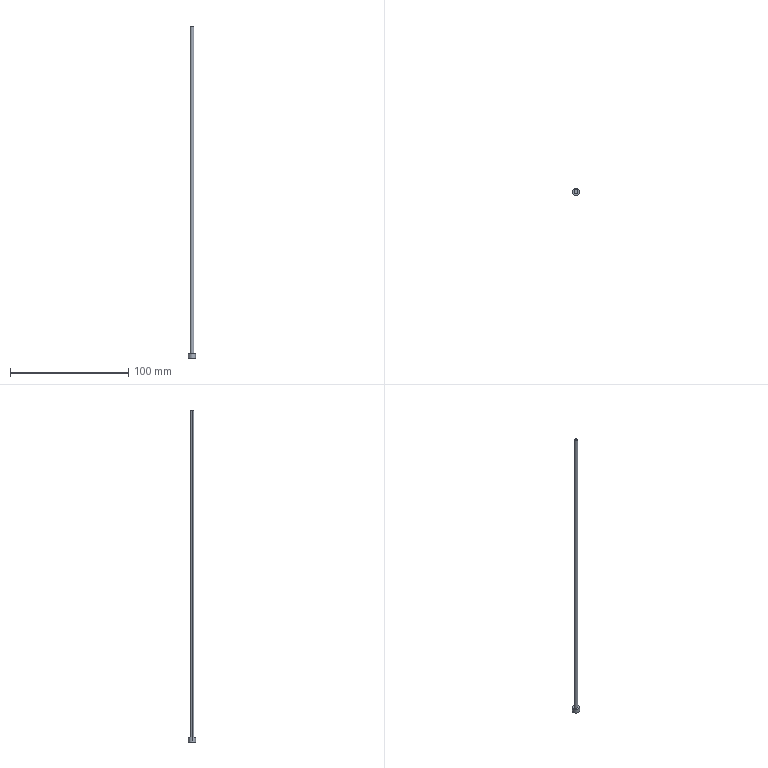Part | Creo | 1 solid | 7 faces | box 6 x 6 x 280.196 mm | volume 2065 mm3 | cylinder 4 | plane 3 | commonest cylinder face diameters 3 x2 6 x2
STEP:
#1=CARTESIAN_POINT('',(-83.5,0.,-292.));
#2=VERTEX_POINT('',#1);
#3=CARTESIAN_POINT('',(-86.5,0.,-292.));
#4=VERTEX_POINT('',#3);
#5=CARTESIAN_POINT('',(-85.,0.,-292.));
#6=DIRECTION('',(0.,0.,-1.));
#7=DIRECTION('',(1.,0.,0.));
#8=AXIS2_PLACEMENT_3D('',#5,#6,#7);
#9=CIRCLE('',#8,1.5);
#10=EDGE_CURVE('',#2,#4,#9,.T.);
#11=ORIENTED_EDGE('',*,*,#10,.T.);
#12=CARTESIAN_POINT('',(-86.5,0.,-15.804));
#13=VERTEX_POINT('',#12);
#14=CARTESIAN_POINT('',(-86.5,0.,-15.804));
#15=DIRECTION('',(0.,0.,-1.));
#16=VECTOR('',#15,276.196);
#17=LINE('',#14,#16);
#18=EDGE_CURVE('',#13,#4,#17,.T.);
#19=ORIENTED_EDGE('',*,*,#18,.F.);
#20=CARTESIAN_POINT('',(-83.5,0.,-15.804));
#21=VERTEX_POINT('',#20);
#22=CARTESIAN_POINT('',(-85.,0.,-15.804));
#23=DIRECTION('',(0.,0.,1.));
#24=DIRECTION('',(-1.,0.,0.));
#25=AXIS2_PLACEMENT_3D('',#22,#23,#24);
#26=CIRCLE('',#25,1.5);
#27=EDGE_CURVE('',#13,#21,#26,.T.);
#28=ORIENTED_EDGE('',*,*,#27,.T.);
#29=CARTESIAN_POINT('',(-83.5,0.,-15.804));
#30=DIRECTION('',(0.,0.,-1.));
#31=VECTOR('',#30,276.196);
#32=LINE('',#29,#31);
#33=EDGE_CURVE('',#21,#2,#32,.T.);
#34=ORIENTED_EDGE('',*,*,#33,.T.);
#35=EDGE_LOOP('',(#11,#19,#28,#34));
#36=FACE_OUTER_BOUND('',#35,.F.);
#37=CARTESIAN_POINT('',(-85.,0.,45.));
#38=DIRECTION('',(0.,0.,-1.));
#39=DIRECTION('',(1.,0.,0.));
#40=AXIS2_PLACEMENT_3D('',#37,#38,#39);
#41=CYLINDRICAL_SURFACE('',#40,1.5);
#42=ADVANCED_FACE('',(#36),#41,.T.);
#43=CARTESIAN_POINT('',(-82.,0.,-292.));
#44=VERTEX_POINT('',#43);
#45=CARTESIAN_POINT('',(-88.,0.,-292.));
#46=VERTEX_POINT('',#45);
#47=CARTESIAN_POINT('',(-85.,0.,-292.));
#48=DIRECTION('',(0.,0.,1.));
#49=DIRECTION('',(1.,0.,0.));
#50=AXIS2_PLACEMENT_3D('',#47,#48,#49);
#51=CIRCLE('',#50,3.);
#52=EDGE_CURVE('',#44,#46,#51,.T.);
#53=ORIENTED_EDGE('',*,*,#52,.F.);
#54=CARTESIAN_POINT('',(-85.,0.,-292.));
#55=DIRECTION('',(0.,0.,1.));
#56=DIRECTION('',(-1.,0.,0.));
#57=AXIS2_PLACEMENT_3D('',#54,#55,#56);
#58=CIRCLE('',#57,3.);
#59=EDGE_CURVE('',#46,#44,#58,.T.);
#60=ORIENTED_EDGE('',*,*,#59,.F.);
#61=EDGE_LOOP('',(#53,#60));
#62=FACE_OUTER_BOUND('',#61,.F.);
#63=ORIENTED_EDGE('',*,*,#10,.F.);
#64=CARTESIAN_POINT('',(-85.,0.,-292.));
#65=DIRECTION('',(0.,0.,-1.));
#66=DIRECTION('',(-1.,0.,0.));
#67=AXIS2_PLACEMENT_3D('',#64,#65,#66);
#68=CIRCLE('',#67,1.5);
#69=EDGE_CURVE('',#4,#2,#68,.T.);
#70=ORIENTED_EDGE('',*,*,#69,.F.);
#71=EDGE_LOOP('',(#63,#70));
#72=FACE_BOUND('',#71,.F.);
#73=CARTESIAN_POINT('',(-85.,0.,-292.));
#74=DIRECTION('',(0.,0.,1.));
#75=DIRECTION('',(-1.,0.,0.));
#76=AXIS2_PLACEMENT_3D('',#73,#74,#75);
#77=PLANE('',#76);
#78=ADVANCED_FACE('',(#62,#72),#77,.T.);
#79=ORIENTED_EDGE('',*,*,#69,.T.);
#80=ORIENTED_EDGE('',*,*,#33,.F.);
#81=CARTESIAN_POINT('',(-85.,0.,-15.804));
#82=DIRECTION('',(0.,0.,1.));
#83=DIRECTION('',(1.,0.,0.));
#84=AXIS2_PLACEMENT_3D('',#81,#82,#83);
#85=CIRCLE('',#84,1.5);
#86=EDGE_CURVE('',#21,#13,#85,.T.);
#87=ORIENTED_EDGE('',*,*,#86,.T.);
#88=ORIENTED_EDGE('',*,*,#18,.T.);
#89=EDGE_LOOP('',(#79,#80,#87,#88));
#90=FACE_OUTER_BOUND('',#89,.F.);
#91=CARTESIAN_POINT('',(-85.,0.,45.));
#92=DIRECTION('',(0.,0.,-1.));
#93=DIRECTION('',(1.,0.,0.));
#94=AXIS2_PLACEMENT_3D('',#91,#92,#93);
#95=CYLINDRICAL_SURFACE('',#94,1.5);
#96=ADVANCED_FACE('',(#90),#95,.T.);
#97=ORIENTED_EDGE('',*,*,#27,.F.);
#98=ORIENTED_EDGE('',*,*,#86,.F.);
#99=EDGE_LOOP('',(#97,#98));
#100=FACE_OUTER_BOUND('',#99,.F.);
#101=CARTESIAN_POINT('',(0.,0.,-15.804));
#102=DIRECTION('',(0.,0.,-1.));
#103=DIRECTION('',(0.,-1.,0.));
#104=AXIS2_PLACEMENT_3D('',#101,#102,#103);
#105=PLANE('',#104);
#106=ADVANCED_FACE('',(#100),#105,.F.);
#107=ORIENTED_EDGE('',*,*,#52,.T.);
#108=CARTESIAN_POINT('',(-88.,0.,-296.));
#109=VERTEX_POINT('',#108);
#110=CARTESIAN_POINT('',(-88.,0.,-296.));
#111=DIRECTION('',(0.,0.,1.));
#112=VECTOR('',#111,4.);
#113=LINE('',#110,#112);
#114=EDGE_CURVE('',#109,#46,#113,.T.);
#115=ORIENTED_EDGE('',*,*,#114,.F.);
#116=CARTESIAN_POINT('',(-82.,0.,-296.));
#117=VERTEX_POINT('',#116);
#118=CARTESIAN_POINT('',(-85.,0.,-296.));
#119=DIRECTION('',(0.,0.,-1.));
#120=DIRECTION('',(-1.,0.,0.));
#121=AXIS2_PLACEMENT_3D('',#118,#119,#120);
#122=CIRCLE('',#121,3.);
#123=EDGE_CURVE('',#109,#117,#122,.T.);
#124=ORIENTED_EDGE('',*,*,#123,.T.);
#125=CARTESIAN_POINT('',(-82.,0.,-296.));
#126=DIRECTION('',(0.,0.,1.));
#127=VECTOR('',#126,4.);
#128=LINE('',#125,#127);
#129=EDGE_CURVE('',#117,#44,#128,.T.);
#130=ORIENTED_EDGE('',*,*,#129,.T.);
#131=EDGE_LOOP('',(#107,#115,#124,#130));
#132=FACE_OUTER_BOUND('',#131,.F.);
#133=CARTESIAN_POINT('',(-85.,0.,-296.));
#134=DIRECTION('',(0.,0.,1.));
#135=DIRECTION('',(-1.,0.,0.));
#136=AXIS2_PLACEMENT_3D('',#133,#134,#135);
#137=CYLINDRICAL_SURFACE('',#136,3.);
#138=ADVANCED_FACE('',(#132),#137,.T.);
#139=ORIENTED_EDGE('',*,*,#59,.T.);
#140=ORIENTED_EDGE('',*,*,#129,.F.);
#141=CARTESIAN_POINT('',(-85.,0.,-296.));
#142=DIRECTION('',(0.,0.,-1.));
#143=DIRECTION('',(1.,0.,0.));
#144=AXIS2_PLACEMENT_3D('',#141,#142,#143);
#145=CIRCLE('',#144,3.);
#146=EDGE_CURVE('',#117,#109,#145,.T.);
#147=ORIENTED_EDGE('',*,*,#146,.T.);
#148=ORIENTED_EDGE('',*,*,#114,.T.);
#149=EDGE_LOOP('',(#139,#140,#147,#148));
#150=FACE_OUTER_BOUND('',#149,.F.);
#151=CARTESIAN_POINT('',(-85.,0.,-296.));
#152=DIRECTION('',(0.,0.,1.));
#153=DIRECTION('',(-1.,0.,0.));
#154=AXIS2_PLACEMENT_3D('',#151,#152,#153);
#155=CYLINDRICAL_SURFACE('',#154,3.);
#156=ADVANCED_FACE('',(#150),#155,.T.);
#157=ORIENTED_EDGE('',*,*,#146,.F.);
#158=ORIENTED_EDGE('',*,*,#123,.F.);
#159=EDGE_LOOP('',(#157,#158));
#160=FACE_OUTER_BOUND('',#159,.F.);
#161=CARTESIAN_POINT('',(-50.,-35.,-296.));
#162=DIRECTION('',(0.,0.,-1.));
#163=DIRECTION('',(-1.,0.,0.));
#164=AXIS2_PLACEMENT_3D('',#161,#162,#163);
#165=PLANE('',#164);
#166=ADVANCED_FACE('',(#160),#165,.T.);
#167=CLOSED_SHELL('',(#42,#78,#96,#106,#138,#156,#166));
#168=MANIFOLD_SOLID_BREP('',#167);
#169=(LENGTH_UNIT()NAMED_UNIT(*)SI_UNIT(.MILLI.,.METRE.));
#170=UNCERTAINTY_MEASURE_WITH_UNIT(LENGTH_MEASURE(0.02803),#169,'','');
#171=(NAMED_UNIT(*)PLANE_ANGLE_UNIT()SI_UNIT($,.RADIAN.));
#172=PLANE_ANGLE_MEASURE_WITH_UNIT(PLANE_ANGLE_MEASURE(0.01745),#171);
#173=(CONVERSION_BASED_UNIT('DEGREE',#172)NAMED_UNIT(*)PLANE_ANGLE_UNIT());
#174=(NAMED_UNIT(*)SI_UNIT($,.STERADIAN.)SOLID_ANGLE_UNIT());
#175=(GEOMETRIC_REPRESENTATION_CONTEXT(3)GLOBAL_UNCERTAINTY_ASSIGNED_CONTEXT((#170))GLOBAL_UNIT_ASSIGNED_CONTEXT((#169,#173,#174))REPRESENTATION_CONTEXT('',''));
#176=ADVANCED_BREP_SHAPE_REPRESENTATION('',(#168),#175);